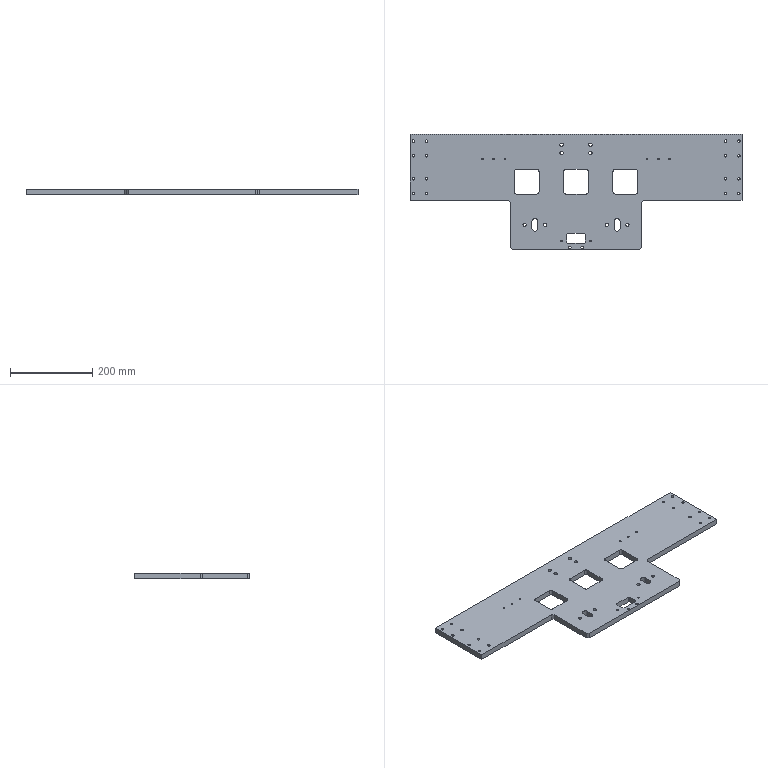Part | SolidWorks | features HoleWzd 5, ICE 4, 3DProfileFeature 3, Chamfer 2, LPattern 2, Extrusion 1, Fillet 1 | 1 solid | 122 faces | box 808 x 280 x 14 mm | volume 2155806 mm3 | cylinder 84 | plane 38 | commonest cylinder face diameters 6 x36 4.2 x16 10 x12 8 x8 8.5 x8 15 x4